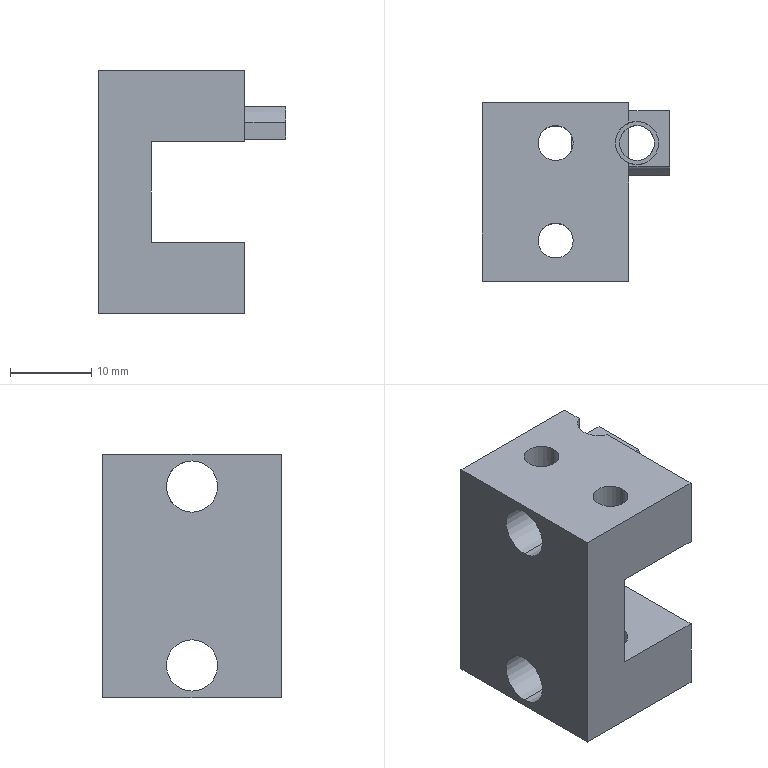Part | SolidWorks | features BaseBody 1 | 1 solid | 36 faces | box 23 x 22 x 30 mm | volume 7166 mm3 | plane 20 | cylinder 16 | commonest cylinder face diameters 4.3 x10 6.3 x4 5.3 x2
STEP:
#1=CARTESIAN_POINT('',(-9.,0.,7.85));
#2=VERTEX_POINT('',#1);
#3=CARTESIAN_POINT('',(-9.,0.,14.15));
#4=VERTEX_POINT('',#3);
#5=CARTESIAN_POINT('',(-9.,0.,11.));
#6=DIRECTION('',(-1.,0.,0.));
#7=DIRECTION('',(0.,0.,-1.));
#8=AXIS2_PLACEMENT_3D('',#5,#6,#7);
#9=CIRCLE('',#8,3.15);
#10=EDGE_CURVE('',#2,#4,#9,.T.);
#11=ORIENTED_EDGE('',*,*,#10,.T.);
#12=CARTESIAN_POINT('',(9.,0.,14.15));
#13=VERTEX_POINT('',#12);
#14=CARTESIAN_POINT('',(-10.,0.,14.15));
#15=DIRECTION('',(1.,0.,0.));
#16=VECTOR('',#15,1000.);
#17=LINE('',#14,#16);
#18=EDGE_CURVE('',#4,#13,#17,.T.);
#19=ORIENTED_EDGE('',*,*,#18,.T.);
#20=CARTESIAN_POINT('',(9.,0.,7.85));
#21=VERTEX_POINT('',#20);
#22=CARTESIAN_POINT('',(9.,0.,11.));
#23=DIRECTION('',(-1.,0.,0.));
#24=DIRECTION('',(0.,0.,-1.));
#25=AXIS2_PLACEMENT_3D('',#22,#23,#24);
#26=CIRCLE('',#25,3.15);
#27=EDGE_CURVE('',#21,#13,#26,.T.);
#28=ORIENTED_EDGE('',*,*,#27,.F.);
#29=CARTESIAN_POINT('',(-10.,0.,7.85));
#30=DIRECTION('',(1.,0.,0.));
#31=VECTOR('',#30,1000.);
#32=LINE('',#29,#31);
#33=EDGE_CURVE('',#2,#21,#32,.T.);
#34=ORIENTED_EDGE('',*,*,#33,.F.);
#35=EDGE_LOOP('',(#11,#19,#28,#34));
#36=FACE_OUTER_BOUND('',#35,.T.);
#37=CARTESIAN_POINT('',(-10.,0.,11.));
#38=DIRECTION('',(1.,0.,0.));
#39=DIRECTION('',(0.,0.,-1.));
#40=AXIS2_PLACEMENT_3D('',#37,#38,#39);
#41=CYLINDRICAL_SURFACE('',#40,3.15);
#42=ADVANCED_FACE('',(#36),#41,.F.);
#43=CARTESIAN_POINT('',(-9.,0.,-14.15));
#44=VERTEX_POINT('',#43);
#45=CARTESIAN_POINT('',(-9.,0.,-7.85));
#46=VERTEX_POINT('',#45);
#47=CARTESIAN_POINT('',(-9.,0.,-11.));
#48=DIRECTION('',(-1.,0.,0.));
#49=DIRECTION('',(0.,0.,-1.));
#50=AXIS2_PLACEMENT_3D('',#47,#48,#49);
#51=CIRCLE('',#50,3.15);
#52=EDGE_CURVE('',#44,#46,#51,.T.);
#53=ORIENTED_EDGE('',*,*,#52,.T.);
#54=CARTESIAN_POINT('',(9.,0.,-7.85));
#55=VERTEX_POINT('',#54);
#56=CARTESIAN_POINT('',(-10.,0.,-7.85));
#57=DIRECTION('',(1.,0.,0.));
#58=VECTOR('',#57,1000.);
#59=LINE('',#56,#58);
#60=EDGE_CURVE('',#46,#55,#59,.T.);
#61=ORIENTED_EDGE('',*,*,#60,.T.);
#62=CARTESIAN_POINT('',(9.,0.,-14.15));
#63=VERTEX_POINT('',#62);
#64=CARTESIAN_POINT('',(9.,0.,-11.));
#65=DIRECTION('',(-1.,0.,0.));
#66=DIRECTION('',(0.,0.,-1.));
#67=AXIS2_PLACEMENT_3D('',#64,#65,#66);
#68=CIRCLE('',#67,3.15);
#69=EDGE_CURVE('',#63,#55,#68,.T.);
#70=ORIENTED_EDGE('',*,*,#69,.F.);
#71=CARTESIAN_POINT('',(-10.,0.,-14.15));
#72=DIRECTION('',(1.,0.,0.));
#73=VECTOR('',#72,1000.);
#74=LINE('',#71,#73);
#75=EDGE_CURVE('',#44,#63,#74,.T.);
#76=ORIENTED_EDGE('',*,*,#75,.F.);
#77=EDGE_LOOP('',(#53,#61,#70,#76));
#78=FACE_OUTER_BOUND('',#77,.T.);
#79=CARTESIAN_POINT('',(-10.,0.,-11.));
#80=DIRECTION('',(1.,0.,0.));
#81=DIRECTION('',(0.,0.,-1.));
#82=AXIS2_PLACEMENT_3D('',#79,#80,#81);
#83=CYLINDRICAL_SURFACE('',#82,3.15);
#84=ADVANCED_FACE('',(#78),#83,.F.);
#85=CARTESIAN_POINT('',(-2.15,6.,6.2));
#86=VERTEX_POINT('',#85);
#87=CARTESIAN_POINT('',(2.15,6.,6.2));
#88=VERTEX_POINT('',#87);
#89=CARTESIAN_POINT('',(0.,6.,6.2));
#90=DIRECTION('',(0.,0.,1.));
#91=DIRECTION('',(1.,0.,0.));
#92=AXIS2_PLACEMENT_3D('',#89,#90,#91);
#93=CIRCLE('',#92,2.15);
#94=EDGE_CURVE('',#86,#88,#93,.T.);
#95=ORIENTED_EDGE('',*,*,#94,.F.);
#96=CARTESIAN_POINT('',(-2.15,6.,15.));
#97=VERTEX_POINT('',#96);
#98=CARTESIAN_POINT('',(-2.15,6.,-16.));
#99=DIRECTION('',(0.,0.,1.));
#100=VECTOR('',#99,1000.);
#101=LINE('',#98,#100);
#102=EDGE_CURVE('',#86,#97,#101,.T.);
#103=ORIENTED_EDGE('',*,*,#102,.T.);
#104=CARTESIAN_POINT('',(2.15,6.,15.));
#105=VERTEX_POINT('',#104);
#106=CARTESIAN_POINT('',(0.,6.,15.));
#107=DIRECTION('',(0.,0.,-1.));
#108=DIRECTION('',(1.,0.,0.));
#109=AXIS2_PLACEMENT_3D('',#106,#107,#108);
#110=CIRCLE('',#109,2.15);
#111=EDGE_CURVE('',#105,#97,#110,.T.);
#112=ORIENTED_EDGE('',*,*,#111,.F.);
#113=CARTESIAN_POINT('',(2.15,6.,10.5));
#114=VERTEX_POINT('',#113);
#115=CARTESIAN_POINT('',(2.15,6.,-16.));
#116=DIRECTION('',(0.,0.,1.));
#117=VECTOR('',#116,1000.);
#118=LINE('',#115,#117);
#119=EDGE_CURVE('',#114,#105,#118,.T.);
#120=ORIENTED_EDGE('',*,*,#119,.F.);
#121=CARTESIAN_POINT('',(2.,5.211,10.5));
#122=VERTEX_POINT('',#121);
#123=CARTESIAN_POINT('',(0.,6.,10.5));
#124=DIRECTION('',(0.,0.,1.));
#125=DIRECTION('',(1.,0.,0.));
#126=AXIS2_PLACEMENT_3D('',#123,#124,#125);
#127=CIRCLE('',#126,2.15);
#128=EDGE_CURVE('',#122,#114,#127,.T.);
#129=ORIENTED_EDGE('',*,*,#128,.F.);
#130=CARTESIAN_POINT('',(2.,5.211,6.5));
#131=VERTEX_POINT('',#130);
#132=CARTESIAN_POINT('',(2.,5.211,-16.));
#133=DIRECTION('',(0.,0.,1.));
#134=VECTOR('',#133,1000.);
#135=LINE('',#132,#134);
#136=EDGE_CURVE('',#131,#122,#135,.T.);
#137=ORIENTED_EDGE('',*,*,#136,.F.);
#138=CARTESIAN_POINT('',(2.15,6.,6.5));
#139=VERTEX_POINT('',#138);
#140=CARTESIAN_POINT('',(0.,6.,6.5));
#141=DIRECTION('',(0.,0.,-1.));
#142=DIRECTION('',(1.,0.,0.));
#143=AXIS2_PLACEMENT_3D('',#140,#141,#142);
#144=CIRCLE('',#143,2.15);
#145=EDGE_CURVE('',#139,#131,#144,.T.);
#146=ORIENTED_EDGE('',*,*,#145,.F.);
#147=CARTESIAN_POINT('',(2.15,6.,-16.));
#148=DIRECTION('',(0.,0.,1.));
#149=VECTOR('',#148,1000.);
#150=LINE('',#147,#149);
#151=EDGE_CURVE('',#88,#139,#150,.T.);
#152=ORIENTED_EDGE('',*,*,#151,.F.);
#153=EDGE_LOOP('',(#95,#103,#112,#120,#129,#137,#146,#152));
#154=FACE_OUTER_BOUND('',#153,.T.);
#155=CARTESIAN_POINT('',(0.,6.,-16.));
#156=DIRECTION('',(0.,0.,1.));
#157=DIRECTION('',(1.,0.,0.));
#158=AXIS2_PLACEMENT_3D('',#155,#156,#157);
#159=CYLINDRICAL_SURFACE('',#158,2.15);
#160=ADVANCED_FACE('',(#154),#159,.F.);
#161=CARTESIAN_POINT('',(-2.15,-6.,6.2));
#162=VERTEX_POINT('',#161);
#163=CARTESIAN_POINT('',(2.15,-6.,6.2));
#164=VERTEX_POINT('',#163);
#165=CARTESIAN_POINT('',(0.,-6.,6.2));
#166=DIRECTION('',(0.,0.,1.));
#167=DIRECTION('',(1.,0.,0.));
#168=AXIS2_PLACEMENT_3D('',#165,#166,#167);
#169=CIRCLE('',#168,2.15);
#170=EDGE_CURVE('',#162,#164,#169,.T.);
#171=ORIENTED_EDGE('',*,*,#170,.F.);
#172=CARTESIAN_POINT('',(-2.15,-6.,15.));
#173=VERTEX_POINT('',#172);
#174=CARTESIAN_POINT('',(-2.15,-6.,-16.));
#175=DIRECTION('',(0.,0.,1.));
#176=VECTOR('',#175,1000.);
#177=LINE('',#174,#176);
#178=EDGE_CURVE('',#162,#173,#177,.T.);
#179=ORIENTED_EDGE('',*,*,#178,.T.);
#180=CARTESIAN_POINT('',(2.15,-6.,15.));
#181=VERTEX_POINT('',#180);
#182=CARTESIAN_POINT('',(0.,-6.,15.));
#183=DIRECTION('',(0.,0.,-1.));
#184=DIRECTION('',(1.,0.,0.));
#185=AXIS2_PLACEMENT_3D('',#182,#183,#184);
#186=CIRCLE('',#185,2.15);
#187=EDGE_CURVE('',#181,#173,#186,.T.);
#188=ORIENTED_EDGE('',*,*,#187,.F.);
#189=CARTESIAN_POINT('',(2.15,-6.,-16.));
#190=DIRECTION('',(0.,0.,1.));
#191=VECTOR('',#190,1000.);
#192=LINE('',#189,#191);
#193=EDGE_CURVE('',#164,#181,#192,.T.);
#194=ORIENTED_EDGE('',*,*,#193,.F.);
#195=EDGE_LOOP('',(#171,#179,#188,#194));
#196=FACE_OUTER_BOUND('',#195,.T.);
#197=CARTESIAN_POINT('',(0.,-6.,-16.));
#198=DIRECTION('',(0.,0.,1.));
#199=DIRECTION('',(1.,0.,0.));
#200=AXIS2_PLACEMENT_3D('',#197,#198,#199);
#201=CYLINDRICAL_SURFACE('',#200,2.15);
#202=ADVANCED_FACE('',(#196),#201,.F.);
#203=CARTESIAN_POINT('',(7.35,6.,9.));
#204=VERTEX_POINT('',#203);
#205=CARTESIAN_POINT('',(12.65,6.,9.));
#206=VERTEX_POINT('',#205);
#207=CARTESIAN_POINT('',(10.,6.,9.));
#208=DIRECTION('',(0.,0.,1.));
#209=DIRECTION('',(1.,0.,0.));
#210=AXIS2_PLACEMENT_3D('',#207,#208,#209);
#211=CIRCLE('',#210,2.65);
#212=EDGE_CURVE('',#204,#206,#211,.T.);
#213=ORIENTED_EDGE('',*,*,#212,.F.);
#214=CARTESIAN_POINT('',(7.35,6.,15.));
#215=VERTEX_POINT('',#214);
#216=CARTESIAN_POINT('',(7.35,6.,9.));
#217=DIRECTION('',(0.,0.,1.));
#218=VECTOR('',#217,1000.);
#219=LINE('',#216,#218);
#220=EDGE_CURVE('',#204,#215,#219,.T.);
#221=ORIENTED_EDGE('',*,*,#220,.T.);
#222=CARTESIAN_POINT('',(9.,3.546,15.));
#223=VERTEX_POINT('',#222);
#224=CARTESIAN_POINT('',(10.,6.,15.));
#225=DIRECTION('',(0.,0.,-1.));
#226=DIRECTION('',(1.,0.,0.));
#227=AXIS2_PLACEMENT_3D('',#224,#225,#226);
#228=CIRCLE('',#227,2.65);
#229=EDGE_CURVE('',#223,#215,#228,.T.);
#230=ORIENTED_EDGE('',*,*,#229,.F.);
#231=CARTESIAN_POINT('',(9.,3.546,10.5));
#232=VERTEX_POINT('',#231);
#233=CARTESIAN_POINT('',(9.,3.546,-15.));
#234=DIRECTION('',(0.,0.,1.));
#235=VECTOR('',#234,1000.);
#236=LINE('',#233,#235);
#237=EDGE_CURVE('',#232,#223,#236,.T.);
#238=ORIENTED_EDGE('',*,*,#237,.F.);
#239=CARTESIAN_POINT('',(12.65,6.,10.5));
#240=VERTEX_POINT('',#239);
#241=CARTESIAN_POINT('',(10.,6.,10.5));
#242=DIRECTION('',(0.,0.,-1.));
#243=DIRECTION('',(1.,0.,0.));
#244=AXIS2_PLACEMENT_3D('',#241,#242,#243);
#245=CIRCLE('',#244,2.65);
#246=EDGE_CURVE('',#240,#232,#245,.T.);
#247=ORIENTED_EDGE('',*,*,#246,.F.);
#248=CARTESIAN_POINT('',(12.65,6.,9.));
#249=DIRECTION('',(0.,0.,1.));
#250=VECTOR('',#249,1000.);
#251=LINE('',#248,#250);
#252=EDGE_CURVE('',#206,#240,#251,.T.);
#253=ORIENTED_EDGE('',*,*,#252,.F.);
#254=EDGE_LOOP('',(#213,#221,#230,#238,#247,#253));
#255=FACE_OUTER_BOUND('',#254,.T.);
#256=CARTESIAN_POINT('',(10.,6.,9.));
#257=DIRECTION('',(0.,0.,1.));
#258=DIRECTION('',(1.,0.,0.));
#259=AXIS2_PLACEMENT_3D('',#256,#257,#258);
#260=CYLINDRICAL_SURFACE('',#259,2.65);
#261=ADVANCED_FACE('',(#255),#260,.F.);
#262=CARTESIAN_POINT('',(2.15,6.,-15.));
#263=VERTEX_POINT('',#262);
#264=CARTESIAN_POINT('',(-2.15,6.,-15.));
#265=VERTEX_POINT('',#264);
#266=CARTESIAN_POINT('',(0.,6.,-15.));
#267=DIRECTION('',(0.,0.,-1.));
#268=DIRECTION('',(1.,0.,0.));
#269=AXIS2_PLACEMENT_3D('',#266,#267,#268);
#270=CIRCLE('',#269,2.15);
#271=EDGE_CURVE('',#263,#265,#270,.T.);
#272=ORIENTED_EDGE('',*,*,#271,.T.);
#273=CARTESIAN_POINT('',(-2.15,6.,-6.2));
#274=VERTEX_POINT('',#273);
#275=CARTESIAN_POINT('',(-2.15,6.,-16.));
#276=DIRECTION('',(0.,0.,1.));
#277=VECTOR('',#276,1000.);
#278=LINE('',#275,#277);
#279=EDGE_CURVE('',#265,#274,#278,.T.);
#280=ORIENTED_EDGE('',*,*,#279,.T.);
#281=CARTESIAN_POINT('',(2.15,6.,-6.2));
#282=VERTEX_POINT('',#281);
#283=CARTESIAN_POINT('',(0.,6.,-6.2));
#284=DIRECTION('',(0.,0.,-1.));
#285=DIRECTION('',(1.,0.,0.));
#286=AXIS2_PLACEMENT_3D('',#283,#284,#285);
#287=CIRCLE('',#286,2.15);
#288=EDGE_CURVE('',#282,#274,#287,.T.);
#289=ORIENTED_EDGE('',*,*,#288,.F.);
#290=CARTESIAN_POINT('',(2.15,6.,-16.));
#291=DIRECTION('',(0.,0.,1.));
#292=VECTOR('',#291,1000.);
#293=LINE('',#290,#292);
#294=EDGE_CURVE('',#263,#282,#293,.T.);
#295=ORIENTED_EDGE('',*,*,#294,.F.);
#296=EDGE_LOOP('',(#272,#280,#289,#295));
#297=FACE_OUTER_BOUND('',#296,.T.);
#298=CARTESIAN_POINT('',(0.,6.,-16.));
#299=DIRECTION('',(0.,0.,1.));
#300=DIRECTION('',(1.,0.,0.));
#301=AXIS2_PLACEMENT_3D('',#298,#299,#300);
#302=CYLINDRICAL_SURFACE('',#301,2.15);
#303=ADVANCED_FACE('',(#297),#302,.F.);
#304=CARTESIAN_POINT('',(2.15,-6.,-15.));
#305=VERTEX_POINT('',#304);
#306=CARTESIAN_POINT('',(-2.15,-6.,-15.));
#307=VERTEX_POINT('',#306);
#308=CARTESIAN_POINT('',(0.,-6.,-15.));
#309=DIRECTION('',(0.,0.,-1.));
#310=DIRECTION('',(1.,0.,0.));
#311=AXIS2_PLACEMENT_3D('',#308,#309,#310);
#312=CIRCLE('',#311,2.15);
#313=EDGE_CURVE('',#305,#307,#312,.T.);
#314=ORIENTED_EDGE('',*,*,#313,.T.);
#315=CARTESIAN_POINT('',(-2.15,-6.,-6.2));
#316=VERTEX_POINT('',#315);
#317=CARTESIAN_POINT('',(-2.15,-6.,-16.));
#318=DIRECTION('',(0.,0.,1.));
#319=VECTOR('',#318,1000.);
#320=LINE('',#317,#319);
#321=EDGE_CURVE('',#307,#316,#320,.T.);
#322=ORIENTED_EDGE('',*,*,#321,.T.);
#323=CARTESIAN_POINT('',(2.15,-6.,-6.2));
#324=VERTEX_POINT('',#323);
#325=CARTESIAN_POINT('',(0.,-6.,-6.2));
#326=DIRECTION('',(0.,0.,-1.));
#327=DIRECTION('',(1.,0.,0.));
#328=AXIS2_PLACEMENT_3D('',#325,#326,#327);
#329=CIRCLE('',#328,2.15);
#330=EDGE_CURVE('',#324,#316,#329,.T.);
#331=ORIENTED_EDGE('',*,*,#330,.F.);
#332=CARTESIAN_POINT('',(2.15,-6.,-16.));
#333=DIRECTION('',(0.,0.,1.));
#334=VECTOR('',#333,1000.);
#335=LINE('',#332,#334);
#336=EDGE_CURVE('',#305,#324,#335,.T.);
#337=ORIENTED_EDGE('',*,*,#336,.F.);
#338=EDGE_LOOP('',(#314,#322,#331,#337));
#339=FACE_OUTER_BOUND('',#338,.T.);
#340=CARTESIAN_POINT('',(0.,-6.,-16.));
#341=DIRECTION('',(0.,0.,1.));
#342=DIRECTION('',(1.,0.,0.));
#343=AXIS2_PLACEMENT_3D('',#340,#341,#342);
#344=CYLINDRICAL_SURFACE('',#343,2.15);
#345=ADVANCED_FACE('',(#339),#344,.F.);
#346=CARTESIAN_POINT('',(9.,4.097,6.2));
#347=VERTEX_POINT('',#346);
#348=CARTESIAN_POINT('',(7.85,6.,6.2));
#349=VERTEX_POINT('',#348);
#350=CARTESIAN_POINT('',(10.,6.,6.2));
#351=DIRECTION('',(0.,0.,-1.));
#352=DIRECTION('',(1.,0.,0.));
#353=AXIS2_PLACEMENT_3D('',#350,#351,#352);
#354=CIRCLE('',#353,2.15);
#355=EDGE_CURVE('',#347,#349,#354,.T.);
#356=ORIENTED_EDGE('',*,*,#355,.T.);
#357=CARTESIAN_POINT('',(7.85,6.,9.));
#358=VERTEX_POINT('',#357);
#359=CARTESIAN_POINT('',(7.85,6.,0.5));
#360=DIRECTION('',(0.,0.,1.));
#361=VECTOR('',#360,1000.);
#362=LINE('',#359,#361);
#363=EDGE_CURVE('',#349,#358,#362,.T.);
#364=ORIENTED_EDGE('',*,*,#363,.T.);
#365=CARTESIAN_POINT('',(12.15,6.,9.));
#366=VERTEX_POINT('',#365);
#367=CARTESIAN_POINT('',(10.,6.,9.));
#368=DIRECTION('',(0.,0.,-1.));
#369=DIRECTION('',(1.,0.,0.));
#370=AXIS2_PLACEMENT_3D('',#367,#368,#369);
#371=CIRCLE('',#370,2.15);
#372=EDGE_CURVE('',#366,#358,#371,.T.);
#373=ORIENTED_EDGE('',*,*,#372,.F.);
#374=CARTESIAN_POINT('',(12.15,6.,6.5));
#375=VERTEX_POINT('',#374);
#376=CARTESIAN_POINT('',(12.15,6.,0.5));
#377=DIRECTION('',(0.,0.,1.));
#378=VECTOR('',#377,1000.);
#379=LINE('',#376,#378);
#380=EDGE_CURVE('',#375,#366,#379,.T.);
#381=ORIENTED_EDGE('',*,*,#380,.F.);
#382=CARTESIAN_POINT('',(9.,4.097,6.5));
#383=VERTEX_POINT('',#382);
#384=CARTESIAN_POINT('',(10.,6.,6.5));
#385=DIRECTION('',(0.,0.,-1.));
#386=DIRECTION('',(1.,0.,0.));
#387=AXIS2_PLACEMENT_3D('',#384,#385,#386);
#388=CIRCLE('',#387,2.15);
#389=EDGE_CURVE('',#375,#383,#388,.T.);
#390=ORIENTED_EDGE('',*,*,#389,.T.);
#391=CARTESIAN_POINT('',(9.,4.097,0.5));
#392=DIRECTION('',(0.,0.,1.));
#393=VECTOR('',#392,1000.);
#394=LINE('',#391,#393);
#395=EDGE_CURVE('',#347,#383,#394,.T.);
#396=ORIENTED_EDGE('',*,*,#395,.F.);
#397=EDGE_LOOP('',(#356,#364,#373,#381,#390,#396));
#398=FACE_OUTER_BOUND('',#397,.T.);
#399=CARTESIAN_POINT('',(10.,6.,0.5));
#400=DIRECTION('',(0.,0.,1.));
#401=DIRECTION('',(1.,0.,0.));
#402=AXIS2_PLACEMENT_3D('',#399,#400,#401);
#403=CYLINDRICAL_SURFACE('',#402,2.15);
#404=ADVANCED_FACE('',(#398),#403,.F.);
#405=ORIENTED_EDGE('',*,*,#10,.F.);
#406=CARTESIAN_POINT('',(-9.,0.,11.));
#407=DIRECTION('',(-1.,0.,0.));
#408=DIRECTION('',(0.,0.,-1.));
#409=AXIS2_PLACEMENT_3D('',#406,#407,#408);
#410=CIRCLE('',#409,3.15);
#411=EDGE_CURVE('',#4,#2,#410,.T.);
#412=ORIENTED_EDGE('',*,*,#411,.F.);
#413=EDGE_LOOP('',(#405,#412));
#414=FACE_BOUND('',#413,.T.);
#415=ORIENTED_EDGE('',*,*,#52,.F.);
#416=CARTESIAN_POINT('',(-9.,0.,-11.));
#417=DIRECTION('',(-1.,0.,0.));
#418=DIRECTION('',(0.,0.,-1.));
#419=AXIS2_PLACEMENT_3D('',#416,#417,#418);
#420=CIRCLE('',#419,3.15);
#421=EDGE_CURVE('',#46,#44,#420,.T.);
#422=ORIENTED_EDGE('',*,*,#421,.F.);
#423=EDGE_LOOP('',(#415,#422));
#424=FACE_BOUND('',#423,.T.);
#425=CARTESIAN_POINT('',(-9.,11.,-15.));
#426=VERTEX_POINT('',#425);
#427=CARTESIAN_POINT('',(-9.,11.,15.));
#428=VERTEX_POINT('',#427);
#429=CARTESIAN_POINT('',(-9.,11.,-15.));
#430=DIRECTION('',(0.,0.,1.));
#431=VECTOR('',#430,1000.);
#432=LINE('',#429,#431);
#433=EDGE_CURVE('',#426,#428,#432,.T.);
#434=ORIENTED_EDGE('',*,*,#433,.F.);
#435=CARTESIAN_POINT('',(-9.,-11.,-15.));
#436=VERTEX_POINT('',#435);
#437=CARTESIAN_POINT('',(-9.,-11.,-15.));
#438=DIRECTION('',(0.,1.,0.));
#439=VECTOR('',#438,1000.);
#440=LINE('',#437,#439);
#441=EDGE_CURVE('',#436,#426,#440,.T.);
#442=ORIENTED_EDGE('',*,*,#441,.F.);
#443=CARTESIAN_POINT('',(-9.,-11.,15.));
#444=VERTEX_POINT('',#443);
#445=CARTESIAN_POINT('',(-9.,-11.,-15.));
#446=DIRECTION('',(0.,0.,-1.));
#447=VECTOR('',#446,1000.);
#448=LINE('',#445,#447);
#449=EDGE_CURVE('',#444,#436,#448,.T.);
#450=ORIENTED_EDGE('',*,*,#449,.F.);
#451=CARTESIAN_POINT('',(-9.,-11.,15.));
#452=DIRECTION('',(0.,-1.,0.));
#453=VECTOR('',#452,1000.);
#454=LINE('',#451,#453);
#455=EDGE_CURVE('',#428,#444,#454,.T.);
#456=ORIENTED_EDGE('',*,*,#455,.F.);
#457=EDGE_LOOP('',(#434,#442,#450,#456));
#458=FACE_OUTER_BOUND('',#457,.T.);
#459=CARTESIAN_POINT('',(-9.,-11.,-15.));
#460=DIRECTION('',(1.,0.,0.));
#461=DIRECTION('',(0.,0.,-1.));
#462=AXIS2_PLACEMENT_3D('',#459,#460,#461);
#463=PLANE('',#462);
#464=ADVANCED_FACE('',(#414,#424,#458),#463,.F.);
#465=ORIENTED_EDGE('',*,*,#18,.F.);
#466=ORIENTED_EDGE('',*,*,#411,.T.);
#467=ORIENTED_EDGE('',*,*,#33,.T.);
#468=CARTESIAN_POINT('',(9.,2.,8.566));
#469=VERTEX_POINT('',#468);
#470=CARTESIAN_POINT('',(9.,0.,11.));
#471=DIRECTION('',(-1.,0.,0.));
#472=DIRECTION('',(0.,0.,-1.));
#473=AXIS2_PLACEMENT_3D('',#470,#471,#472);
#474=CIRCLE('',#473,3.15);
#475=EDGE_CURVE('',#469,#21,#474,.T.);
#476=ORIENTED_EDGE('',*,*,#475,.F.);
#477=CARTESIAN_POINT('',(14.,2.,8.566));
#478=VERTEX_POINT('',#477);
#479=CARTESIAN_POINT('',(-10.,2.,8.566));
#480=DIRECTION('',(-1.,0.,0.));
#481=VECTOR('',#480,1000.);
#482=LINE('',#479,#481);
#483=EDGE_CURVE('',#478,#469,#482,.T.);
#484=ORIENTED_EDGE('',*,*,#483,.F.);
#485=CARTESIAN_POINT('',(14.,3.11,10.5));
#486=VERTEX_POINT('',#485);
#487=CARTESIAN_POINT('',(14.,0.,11.));
#488=DIRECTION('',(-1.,0.,0.));
#489=DIRECTION('',(0.,0.,-1.));
#490=AXIS2_PLACEMENT_3D('',#487,#488,#489);
#491=CIRCLE('',#490,3.15);
#492=EDGE_CURVE('',#486,#478,#491,.T.);
#493=ORIENTED_EDGE('',*,*,#492,.F.);
#494=CARTESIAN_POINT('',(9.,3.11,10.5));
#495=VERTEX_POINT('',#494);
#496=CARTESIAN_POINT('',(-10.,3.11,10.5));
#497=DIRECTION('',(1.,0.,0.));
#498=VECTOR('',#497,1000.);
#499=LINE('',#496,#498);
#500=EDGE_CURVE('',#495,#486,#499,.T.);
#501=ORIENTED_EDGE('',*,*,#500,.F.);
#502=CARTESIAN_POINT('',(9.,0.,11.));
#503=DIRECTION('',(-1.,0.,0.));
#504=DIRECTION('',(0.,0.,-1.));
#505=AXIS2_PLACEMENT_3D('',#502,#503,#504);
#506=CIRCLE('',#505,3.15);
#507=EDGE_CURVE('',#13,#495,#506,.T.);
#508=ORIENTED_EDGE('',*,*,#507,.F.);
#509=EDGE_LOOP('',(#465,#466,#467,#476,#484,#493,#501,#508));
#510=FACE_OUTER_BOUND('',#509,.T.);
#511=CARTESIAN_POINT('',(-10.,0.,11.));
#512=DIRECTION('',(1.,0.,0.));
#513=DIRECTION('',(0.,0.,-1.));
#514=AXIS2_PLACEMENT_3D('',#511,#512,#513);
#515=CYLINDRICAL_SURFACE('',#514,3.15);
#516=ADVANCED_FACE('',(#510),#515,.F.);
#517=ORIENTED_EDGE('',*,*,#60,.F.);
#518=ORIENTED_EDGE('',*,*,#421,.T.);
#519=ORIENTED_EDGE('',*,*,#75,.T.);
#520=CARTESIAN_POINT('',(9.,0.,-11.));
#521=DIRECTION('',(-1.,0.,0.));
#522=DIRECTION('',(0.,0.,-1.));
#523=AXIS2_PLACEMENT_3D('',#520,#521,#522);
#524=CIRCLE('',#523,3.15);
#525=EDGE_CURVE('',#55,#63,#524,.T.);
#526=ORIENTED_EDGE('',*,*,#525,.F.);
#527=EDGE_LOOP('',(#517,#518,#519,#526));
#528=FACE_OUTER_BOUND('',#527,.T.);
#529=CARTESIAN_POINT('',(-10.,0.,-11.));
#530=DIRECTION('',(1.,0.,0.));
#531=DIRECTION('',(0.,0.,-1.));
#532=AXIS2_PLACEMENT_3D('',#529,#530,#531);
#533=CYLINDRICAL_SURFACE('',#532,3.15);
#534=ADVANCED_FACE('',(#528),#533,.F.);
#535=ORIENTED_EDGE('',*,*,#111,.T.);
#536=CARTESIAN_POINT('',(0.,6.,15.));
#537=DIRECTION('',(0.,0.,-1.));
#538=DIRECTION('',(1.,0.,0.));
#539=AXIS2_PLACEMENT_3D('',#536,#537,#538);
#540=CIRCLE('',#539,2.15);
#541=EDGE_CURVE('',#97,#105,#540,.T.);
#542=ORIENTED_EDGE('',*,*,#541,.T.);
#543=EDGE_LOOP('',(#535,#542));
#544=FACE_BOUND('',#543,.T.);
#545=ORIENTED_EDGE('',*,*,#187,.T.);
#546=CARTESIAN_POINT('',(0.,-6.,15.));
#547=DIRECTION('',(0.,0.,-1.));
#548=DIRECTION('',(1.,0.,0.));
#549=AXIS2_PLACEMENT_3D('',#546,#547,#548);
#550=CIRCLE('',#549,2.15);
#551=EDGE_CURVE('',#173,#181,#550,.T.);
#552=ORIENTED_EDGE('',*,*,#551,.T.);
#553=EDGE_LOOP('',(#545,#552));
#554=FACE_BOUND('',#553,.T.);
#555=ORIENTED_EDGE('',*,*,#229,.T.);
#556=CARTESIAN_POINT('',(9.,8.454,15.));
#557=VERTEX_POINT('',#556);
#558=CARTESIAN_POINT('',(10.,6.,15.));
#559=DIRECTION('',(0.,0.,-1.));
#560=DIRECTION('',(1.,0.,0.));
#561=AXIS2_PLACEMENT_3D('',#558,#559,#560);
#562=CIRCLE('',#561,2.65);
#563=EDGE_CURVE('',#215,#557,#562,.T.);
#564=ORIENTED_EDGE('',*,*,#563,.T.);
#565=CARTESIAN_POINT('',(9.,11.,15.));
#566=VERTEX_POINT('',#565);
#567=CARTESIAN_POINT('',(9.,-11.,15.));
#568=DIRECTION('',(0.,1.,0.));
#569=VECTOR('',#568,1000.);
#570=LINE('',#567,#569);
#571=EDGE_CURVE('',#557,#566,#570,.T.);
#572=ORIENTED_EDGE('',*,*,#571,.T.);
#573=CARTESIAN_POINT('',(-9.,11.,15.));
#574=DIRECTION('',(-1.,0.,0.));
#575=VECTOR('',#574,1000.);
#576=LINE('',#573,#575);
#577=EDGE_CURVE('',#566,#428,#576,.T.);
#578=ORIENTED_EDGE('',*,*,#577,.T.);
#579=ORIENTED_EDGE('',*,*,#455,.T.);
#580=CARTESIAN_POINT('',(9.,-11.,15.));
#581=VERTEX_POINT('',#580);
#582=CARTESIAN_POINT('',(-9.,-11.,15.));
#583=DIRECTION('',(1.,0.,0.));
#584=VECTOR('',#583,1000.);
#585=LINE('',#582,#584);
#586=EDGE_CURVE('',#444,#581,#585,.T.);
#587=ORIENTED_EDGE('',*,*,#586,.T.);
#588=CARTESIAN_POINT('',(9.,-11.,15.));
#589=DIRECTION('',(0.,1.,0.));
#590=VECTOR('',#589,1000.);
#591=LINE('',#588,#590);
#592=EDGE_CURVE('',#581,#223,#591,.T.);
#593=ORIENTED_EDGE('',*,*,#592,.T.);
#594=EDGE_LOOP('',(#555,#564,#572,#578,#579,#587,#593));
#595=FACE_OUTER_BOUND('',#594,.T.);
#596=CARTESIAN_POINT('',(-9.,-11.,15.));
#597=DIRECTION('',(0.,0.,1.));
#598=DIRECTION('',(1.,0.,0.));
#599=AXIS2_PLACEMENT_3D('',#596,#597,#598);
#600=PLANE('',#599);
#601=ADVANCED_FACE('',(#544,#554,#595),#600,.T.);
#602=CARTESIAN_POINT('',(-2.5,11.,6.2));
#603=VERTEX_POINT('',#602);
#604=CARTESIAN_POINT('',(-2.5,11.,-6.2));
#605=VERTEX_POINT('',#604);
#606=CARTESIAN_POINT('',(-2.5,11.,-15.));
#607=DIRECTION('',(0.,0.,-1.));
#608=VECTOR('',#607,1000.);
#609=LINE('',#606,#608);
#610=EDGE_CURVE('',#603,#605,#609,.T.);
#611=ORIENTED_EDGE('',*,*,#610,.T.);
#612=CARTESIAN_POINT('',(9.,11.,-6.2));
#613=VERTEX_POINT('',#612);
#614=CARTESIAN_POINT('',(-9.,11.,-6.2));
#615=DIRECTION('',(1.,0.,0.));
#616=VECTOR('',#615,1000.);
#617=LINE('',#614,#616);
#618=EDGE_CURVE('',#605,#613,#617,.T.);
#619=ORIENTED_EDGE('',*,*,#618,.T.);
#620=CARTESIAN_POINT('',(9.,11.,-15.));
#621=VERTEX_POINT('',#620);
#622=CARTESIAN_POINT('',(9.,11.,-15.));
#623=DIRECTION('',(0.,0.,-1.));
#624=VECTOR('',#623,1000.);
#625=LINE('',#622,#624);
#626=EDGE_CURVE('',#613,#621,#625,.T.);
#627=ORIENTED_EDGE('',*,*,#626,.T.);
#628=CARTESIAN_POINT('',(-9.,11.,-15.));
#629=DIRECTION('',(-1.,0.,0.));
#630=VECTOR('',#629,1000.);
#631=LINE('',#628,#630);
#632=EDGE_CURVE('',#621,#426,#631,.T.);
#633=ORIENTED_EDGE('',*,*,#632,.T.);
#634=ORIENTED_EDGE('',*,*,#433,.T.);
#635=ORIENTED_EDGE('',*,*,#577,.F.);
#636=CARTESIAN_POINT('',(9.,11.,6.2));
#637=VERTEX_POINT('',#636);
#638=CARTESIAN_POINT('',(9.,11.,-15.));
#639=DIRECTION('',(0.,0.,-1.));
#640=VECTOR('',#639,1000.);
#641=LINE('',#638,#640);
#642=EDGE_CURVE('',#566,#637,#641,.T.);
#643=ORIENTED_EDGE('',*,*,#642,.T.);
#644=CARTESIAN_POINT('',(-9.,11.,6.2));
#645=DIRECTION('',(-1.,0.,0.));
#646=VECTOR('',#645,1000.);
#647=LINE('',#644,#646);
#648=EDGE_CURVE('',#637,#603,#647,.T.);
#649=ORIENTED_EDGE('',*,*,#648,.T.);
#650=EDGE_LOOP('',(#611,#619,#627,#633,#634,#635,#643,#649));
#651=FACE_OUTER_BOUND('',#650,.T.);
#652=CARTESIAN_POINT('',(-9.,11.,-15.));
#653=DIRECTION('',(0.,1.,0.));
#654=DIRECTION('',(0.,0.,1.));
#655=AXIS2_PLACEMENT_3D('',#652,#653,#654);
#656=PLANE('',#655);
#657=ADVANCED_FACE('',(#651),#656,.T.);
#658=ORIENTED_EDGE('',*,*,#271,.F.);
#659=CARTESIAN_POINT('',(0.,6.,-15.));
#660=DIRECTION('',(0.,0.,-1.));
#661=DIRECTION('',(1.,0.,0.));
#662=AXIS2_PLACEMENT_3D('',#659,#660,#661);
#663=CIRCLE('',#662,2.15);
#664=EDGE_CURVE('',#265,#263,#663,.T.);
#665=ORIENTED_EDGE('',*,*,#664,.F.);
#666=EDGE_LOOP('',(#658,#665));
#667=FACE_BOUND('',#666,.T.);
#668=ORIENTED_EDGE('',*,*,#313,.F.);
#669=CARTESIAN_POINT('',(0.,-6.,-15.));
#670=DIRECTION('',(0.,0.,-1.));
#671=DIRECTION('',(1.,0.,0.));
#672=AXIS2_PLACEMENT_3D('',#669,#670,#671);
#673=CIRCLE('',#672,2.15);
#674=EDGE_CURVE('',#307,#305,#673,.T.);
#675=ORIENTED_EDGE('',*,*,#674,.F.);
#676=EDGE_LOOP('',(#668,#675));
#677=FACE_BOUND('',#676,.T.);
#678=CARTESIAN_POINT('',(9.,-11.,-15.));
#679=VERTEX_POINT('',#678);
#680=CARTESIAN_POINT('',(9.,-11.,-15.));
#681=DIRECTION('',(0.,1.,0.));
#682=VECTOR('',#681,1000.);
#683=LINE('',#680,#682);
#684=EDGE_CURVE('',#679,#621,#683,.T.);
#685=ORIENTED_EDGE('',*,*,#684,.F.);
#686=CARTESIAN_POINT('',(-9.,-11.,-15.));
#687=DIRECTION('',(1.,0.,0.));
#688=VECTOR('',#687,1000.);
#689=LINE('',#686,#688);
#690=EDGE_CURVE('',#436,#679,#689,.T.);
#691=ORIENTED_EDGE('',*,*,#690,.F.);
#692=ORIENTED_EDGE('',*,*,#441,.T.);
#693=ORIENTED_EDGE('',*,*,#632,.F.);
#694=EDGE_LOOP('',(#685,#691,#692,#693));
#695=FACE_OUTER_BOUND('',#694,.T.);
#696=CARTESIAN_POINT('',(-9.,-11.,-15.));
#697=DIRECTION('',(0.,0.,1.));
#698=DIRECTION('',(1.,0.,0.));
#699=AXIS2_PLACEMENT_3D('',#696,#697,#698);
#700=PLANE('',#699);
#701=ADVANCED_FACE('',(#667,#677,#695),#700,.F.);
#702=CARTESIAN_POINT('',(-2.5,-11.,6.2));
#703=VERTEX_POINT('',#702);
#704=CARTESIAN_POINT('',(-2.5,-11.,-6.2));
#705=VERTEX_POINT('',#704);
#706=CARTESIAN_POINT('',(-2.5,-11.,-15.));
#707=DIRECTION('',(0.,0.,-1.));
#708=VECTOR('',#707,1000.);
#709=LINE('',#706,#708);
#710=EDGE_CURVE('',#703,#705,#709,.T.);
#711=ORIENTED_EDGE('',*,*,#710,.F.);
#712=CARTESIAN_POINT('',(9.,-11.,6.2));
#713=VERTEX_POINT('',#712);
#714=CARTESIAN_POINT('',(-9.,-11.,6.2));
#715=DIRECTION('',(-1.,0.,0.));
#716=VECTOR('',#715,1000.);
#717=LINE('',#714,#716);
#718=EDGE_CURVE('',#713,#703,#717,.T.);
#719=ORIENTED_EDGE('',*,*,#718,.F.);
#720=CARTESIAN_POINT('',(9.,-11.,-15.));
#721=DIRECTION('',(0.,0.,-1.));
#722=VECTOR('',#721,1000.);
#723=LINE('',#720,#722);
#724=EDGE_CURVE('',#581,#713,#723,.T.);
#725=ORIENTED_EDGE('',*,*,#724,.F.);
#726=ORIENTED_EDGE('',*,*,#586,.F.);
#727=ORIENTED_EDGE('',*,*,#449,.T.);
#728=ORIENTED_EDGE('',*,*,#690,.T.);
#729=CARTESIAN_POINT('',(9.,-11.,-6.2));
#730=VERTEX_POINT('',#729);
#731=CARTESIAN_POINT('',(9.,-11.,-15.));
#732=DIRECTION('',(0.,0.,-1.));
#733=VECTOR('',#732,1000.);
#734=LINE('',#731,#733);
#735=EDGE_CURVE('',#730,#679,#734,.T.);
#736=ORIENTED_EDGE('',*,*,#735,.F.);
#737=CARTESIAN_POINT('',(-9.,-11.,-6.2));
#738=DIRECTION('',(1.,0.,0.));
#739=VECTOR('',#738,1000.);
#740=LINE('',#737,#739);
#741=EDGE_CURVE('',#705,#730,#740,.T.);
#742=ORIENTED_EDGE('',*,*,#741,.F.);
#743=EDGE_LOOP('',(#711,#719,#725,#726,#727,#728,#736,#742));
#744=FACE_OUTER_BOUND('',#743,.T.);
#745=CARTESIAN_POINT('',(-9.,-11.,-15.));
#746=DIRECTION('',(0.,1.,0.));
#747=DIRECTION('',(0.,0.,1.));
#748=AXIS2_PLACEMENT_3D('',#745,#746,#747);
#749=PLANE('',#748);
#750=ADVANCED_FACE('',(#744),#749,.F.);
#751=ORIENTED_EDGE('',*,*,#237,.T.);
#752=ORIENTED_EDGE('',*,*,#592,.F.);
#753=ORIENTED_EDGE('',*,*,#724,.T.);
#754=CARTESIAN_POINT('',(9.,-11.,6.2));
#755=DIRECTION('',(0.,1.,0.));
#756=VECTOR('',#755,1000.);
#757=LINE('',#754,#756);
#758=EDGE_CURVE('',#713,#347,#757,.T.);
#759=ORIENTED_EDGE('',*,*,#758,.T.);
#760=ORIENTED_EDGE('',*,*,#395,.T.);
#761=CARTESIAN_POINT('',(9.,2.,6.5));
#762=VERTEX_POINT('',#761);
#763=CARTESIAN_POINT('',(9.,-11.,6.5));
#764=DIRECTION('',(0.,-1.,0.));
#765=VECTOR('',#764,1000.);
#766=LINE('',#763,#765);
#767=EDGE_CURVE('',#383,#762,#766,.T.);
#768=ORIENTED_EDGE('',*,*,#767,.T.);
#769=CARTESIAN_POINT('',(9.,2.,-15.));
#770=DIRECTION('',(0.,0.,1.));
#771=VECTOR('',#770,1000.);
#772=LINE('',#769,#771);
#773=EDGE_CURVE('',#762,#469,#772,.T.);
#774=ORIENTED_EDGE('',*,*,#773,.T.);
#775=ORIENTED_EDGE('',*,*,#475,.T.);
#776=ORIENTED_EDGE('',*,*,#27,.T.);
#777=ORIENTED_EDGE('',*,*,#507,.T.);
#778=CARTESIAN_POINT('',(9.,-11.,10.5));
#779=DIRECTION('',(0.,1.,0.));
#780=VECTOR('',#779,1000.);
#781=LINE('',#778,#780);
#782=EDGE_CURVE('',#495,#232,#781,.T.);
#783=ORIENTED_EDGE('',*,*,#782,.T.);
#784=EDGE_LOOP('',(#751,#752,#753,#759,#760,#768,#774,#775,#776,#777,#783));
#785=FACE_OUTER_BOUND('',#784,.T.);
#786=CARTESIAN_POINT('',(9.,-11.,-15.));
#787=DIRECTION('',(1.,0.,0.));
#788=DIRECTION('',(0.,0.,-1.));
#789=AXIS2_PLACEMENT_3D('',#786,#787,#788);
#790=PLANE('',#789);
#791=ADVANCED_FACE('',(#785),#790,.T.);
#792=ORIENTED_EDGE('',*,*,#483,.T.);
#793=ORIENTED_EDGE('',*,*,#773,.F.);
#794=CARTESIAN_POINT('',(14.,2.,6.5));
#795=VERTEX_POINT('',#794);
#796=CARTESIAN_POINT('',(2.,2.,6.5));
#797=DIRECTION('',(-1.,0.,0.));
#798=VECTOR('',#797,1000.);
#799=LINE('',#796,#798);
#800=EDGE_CURVE('',#795,#762,#799,.T.);
#801=ORIENTED_EDGE('',*,*,#800,.F.);
#802=CARTESIAN_POINT('',(14.,2.,6.5));
#803=DIRECTION('',(0.,0.,-1.));
#804=VECTOR('',#803,1000.);
#805=LINE('',#802,#804);
#806=EDGE_CURVE('',#478,#795,#805,.T.);
#807=ORIENTED_EDGE('',*,*,#806,.F.);
#808=EDGE_LOOP('',(#792,#793,#801,#807));
#809=FACE_OUTER_BOUND('',#808,.T.);
#810=CARTESIAN_POINT('',(2.,2.,6.5));
#811=DIRECTION('',(0.,1.,0.));
#812=DIRECTION('',(0.,0.,1.));
#813=AXIS2_PLACEMENT_3D('',#810,#811,#812);
#814=PLANE('',#813);
#815=ADVANCED_FACE('',(#809),#814,.F.);
#816=CARTESIAN_POINT('',(14.,10.,10.5));
#817=VERTEX_POINT('',#816);
#818=CARTESIAN_POINT('',(14.,2.,10.5));
#819=DIRECTION('',(0.,-1.,0.));
#820=VECTOR('',#819,1000.);
#821=LINE('',#818,#820);
#822=EDGE_CURVE('',#817,#486,#821,.T.);
#823=ORIENTED_EDGE('',*,*,#822,.T.);
#824=ORIENTED_EDGE('',*,*,#492,.T.);
#825=ORIENTED_EDGE('',*,*,#806,.T.);
#826=CARTESIAN_POINT('',(14.,10.,6.5));
#827=VERTEX_POINT('',#826);
#828=CARTESIAN_POINT('',(14.,2.,6.5));
#829=DIRECTION('',(0.,1.,0.));
#830=VECTOR('',#829,1000.);
#831=LINE('',#828,#830);
#832=EDGE_CURVE('',#795,#827,#831,.T.);
#833=ORIENTED_EDGE('',*,*,#832,.T.);
#834=CARTESIAN_POINT('',(14.,10.,6.5));
#835=DIRECTION('',(0.,0.,1.));
#836=VECTOR('',#835,1000.);
#837=LINE('',#834,#836);
#838=EDGE_CURVE('',#827,#817,#837,.T.);
#839=ORIENTED_EDGE('',*,*,#838,.T.);
#840=EDGE_LOOP('',(#823,#824,#825,#833,#839));
#841=FACE_OUTER_BOUND('',#840,.T.);
#842=CARTESIAN_POINT('',(14.,2.,6.5));
#843=DIRECTION('',(1.,0.,0.));
#844=DIRECTION('',(0.,0.,-1.));
#845=AXIS2_PLACEMENT_3D('',#842,#843,#844);
#846=PLANE('',#845);
#847=ADVANCED_FACE('',(#841),#846,.T.);
#848=ORIENTED_EDGE('',*,*,#500,.T.);
#849=ORIENTED_EDGE('',*,*,#822,.F.);
#850=CARTESIAN_POINT('',(9.,10.,10.5));
#851=VERTEX_POINT('',#850);
#852=CARTESIAN_POINT('',(2.,10.,10.5));
#853=DIRECTION('',(-1.,0.,0.));
#854=VECTOR('',#853,1000.);
#855=LINE('',#852,#854);
#856=EDGE_CURVE('',#817,#851,#855,.T.);
#857=ORIENTED_EDGE('',*,*,#856,.T.);
#858=CARTESIAN_POINT('',(9.,8.454,10.5));
#859=VERTEX_POINT('',#858);
#860=CARTESIAN_POINT('',(9.,2.,10.5));
#861=DIRECTION('',(0.,-1.,0.));
#862=VECTOR('',#861,1000.);
#863=LINE('',#860,#862);
#864=EDGE_CURVE('',#851,#859,#863,.T.);
#865=ORIENTED_EDGE('',*,*,#864,.T.);
#866=CARTESIAN_POINT('',(10.,6.,10.5));
#867=DIRECTION('',(0.,0.,-1.));
#868=DIRECTION('',(1.,0.,0.));
#869=AXIS2_PLACEMENT_3D('',#866,#867,#868);
#870=CIRCLE('',#869,2.65);
#871=EDGE_CURVE('',#859,#240,#870,.T.);
#872=ORIENTED_EDGE('',*,*,#871,.T.);
#873=ORIENTED_EDGE('',*,*,#246,.T.);
#874=ORIENTED_EDGE('',*,*,#782,.F.);
#875=EDGE_LOOP('',(#848,#849,#857,#865,#872,#873,#874));
#876=FACE_OUTER_BOUND('',#875,.T.);
#877=CARTESIAN_POINT('',(2.,2.,10.5));
#878=DIRECTION('',(0.,0.,1.));
#879=DIRECTION('',(1.,0.,0.));
#880=AXIS2_PLACEMENT_3D('',#877,#878,#879);
#881=PLANE('',#880);
#882=ADVANCED_FACE('',(#876),#881,.T.);
#883=ORIENTED_EDGE('',*,*,#69,.T.);
#884=ORIENTED_EDGE('',*,*,#525,.T.);
#885=EDGE_LOOP('',(#883,#884));
#886=FACE_BOUND('',#885,.T.);
#887=ORIENTED_EDGE('',*,*,#626,.F.);
#888=CARTESIAN_POINT('',(9.,-11.,-6.2));
#889=DIRECTION('',(0.,-1.,0.));
#890=VECTOR('',#889,1000.);
#891=LINE('',#888,#890);
#892=EDGE_CURVE('',#613,#730,#891,.T.);
#893=ORIENTED_EDGE('',*,*,#892,.T.);
#894=ORIENTED_EDGE('',*,*,#735,.T.);
#895=ORIENTED_EDGE('',*,*,#684,.T.);
#896=EDGE_LOOP('',(#887,#893,#894,#895));
#897=FACE_OUTER_BOUND('',#896,.T.);
#898=CARTESIAN_POINT('',(9.,-11.,-15.));
#899=DIRECTION('',(1.,0.,0.));
#900=DIRECTION('',(0.,0.,-1.));
#901=AXIS2_PLACEMENT_3D('',#898,#899,#900);
#902=PLANE('',#901);
#903=ADVANCED_FACE('',(#886,#897),#902,.T.);
#904=ORIENTED_EDGE('',*,*,#102,.F.);
#905=CARTESIAN_POINT('',(0.,6.,6.2));
#906=DIRECTION('',(0.,0.,1.));
#907=DIRECTION('',(1.,0.,0.));
#908=AXIS2_PLACEMENT_3D('',#905,#906,#907);
#909=CIRCLE('',#908,2.15);
#910=EDGE_CURVE('',#88,#86,#909,.T.);
#911=ORIENTED_EDGE('',*,*,#910,.F.);
#912=ORIENTED_EDGE('',*,*,#151,.T.);
#913=CARTESIAN_POINT('',(2.,6.789,6.5));
#914=VERTEX_POINT('',#913);
#915=CARTESIAN_POINT('',(0.,6.,6.5));
#916=DIRECTION('',(0.,0.,-1.));
#917=DIRECTION('',(1.,0.,0.));
#918=AXIS2_PLACEMENT_3D('',#915,#916,#917);
#919=CIRCLE('',#918,2.15);
#920=EDGE_CURVE('',#914,#139,#919,.T.);
#921=ORIENTED_EDGE('',*,*,#920,.F.);
#922=CARTESIAN_POINT('',(2.,6.789,10.5));
#923=VERTEX_POINT('',#922);
#924=CARTESIAN_POINT('',(2.,6.789,-16.));
#925=DIRECTION('',(0.,0.,-1.));
#926=VECTOR('',#925,1000.);
#927=LINE('',#924,#926);
#928=EDGE_CURVE('',#923,#914,#927,.T.);
#929=ORIENTED_EDGE('',*,*,#928,.F.);
#930=CARTESIAN_POINT('',(0.,6.,10.5));
#931=DIRECTION('',(0.,0.,1.));
#932=DIRECTION('',(1.,0.,0.));
#933=AXIS2_PLACEMENT_3D('',#930,#931,#932);
#934=CIRCLE('',#933,2.15);
#935=EDGE_CURVE('',#114,#923,#934,.T.);
#936=ORIENTED_EDGE('',*,*,#935,.F.);
#937=ORIENTED_EDGE('',*,*,#119,.T.);
#938=ORIENTED_EDGE('',*,*,#541,.F.);
#939=EDGE_LOOP('',(#904,#911,#912,#921,#929,#936,#937,#938));
#940=FACE_OUTER_BOUND('',#939,.T.);
#941=CARTESIAN_POINT('',(0.,6.,-16.));
#942=DIRECTION('',(0.,0.,1.));
#943=DIRECTION('',(1.,0.,0.));
#944=AXIS2_PLACEMENT_3D('',#941,#942,#943);
#945=CYLINDRICAL_SURFACE('',#944,2.15);
#946=ADVANCED_FACE('',(#940),#945,.F.);
#947=ORIENTED_EDGE('',*,*,#178,.F.);
#948=CARTESIAN_POINT('',(0.,-6.,6.2));
#949=DIRECTION('',(0.,0.,1.));
#950=DIRECTION('',(1.,0.,0.));
#951=AXIS2_PLACEMENT_3D('',#948,#949,#950);
#952=CIRCLE('',#951,2.15);
#953=EDGE_CURVE('',#164,#162,#952,.T.);
#954=ORIENTED_EDGE('',*,*,#953,.F.);
#955=ORIENTED_EDGE('',*,*,#193,.T.);
#956=ORIENTED_EDGE('',*,*,#551,.F.);
#957=EDGE_LOOP('',(#947,#954,#955,#956));
#958=FACE_OUTER_BOUND('',#957,.T.);
#959=CARTESIAN_POINT('',(0.,-6.,-16.));
#960=DIRECTION('',(0.,0.,1.));
#961=DIRECTION('',(1.,0.,0.));
#962=AXIS2_PLACEMENT_3D('',#959,#960,#961);
#963=CYLINDRICAL_SURFACE('',#962,2.15);
#964=ADVANCED_FACE('',(#958),#963,.F.);
#965=CARTESIAN_POINT('',(9.,10.,6.5));
#966=VERTEX_POINT('',#965);
#967=CARTESIAN_POINT('',(9.,10.,-15.));
#968=DIRECTION('',(0.,0.,-1.));
#969=VECTOR('',#968,1000.);
#970=LINE('',#967,#969);
#971=EDGE_CURVE('',#851,#966,#970,.T.);
#972=ORIENTED_EDGE('',*,*,#971,.T.);
#973=CARTESIAN_POINT('',(9.,7.903,6.5));
#974=VERTEX_POINT('',#973);
#975=CARTESIAN_POINT('',(9.,-11.,6.5));
#976=DIRECTION('',(0.,-1.,0.));
#977=VECTOR('',#976,1000.);
#978=LINE('',#975,#977);
#979=EDGE_CURVE('',#966,#974,#978,.T.);
#980=ORIENTED_EDGE('',*,*,#979,.T.);
#981=CARTESIAN_POINT('',(9.,7.903,6.2));
#982=VERTEX_POINT('',#981);
#983=CARTESIAN_POINT('',(9.,7.903,0.5));
#984=DIRECTION('',(0.,0.,-1.));
#985=VECTOR('',#984,1000.);
#986=LINE('',#983,#985);
#987=EDGE_CURVE('',#974,#982,#986,.T.);
#988=ORIENTED_EDGE('',*,*,#987,.T.);
#989=CARTESIAN_POINT('',(9.,-11.,6.2));
#990=DIRECTION('',(0.,1.,0.));
#991=VECTOR('',#990,1000.);
#992=LINE('',#989,#991);
#993=EDGE_CURVE('',#982,#637,#992,.T.);
#994=ORIENTED_EDGE('',*,*,#993,.T.);
#995=ORIENTED_EDGE('',*,*,#642,.F.);
#996=ORIENTED_EDGE('',*,*,#571,.F.);
#997=CARTESIAN_POINT('',(9.,8.454,-15.));
#998=DIRECTION('',(0.,0.,-1.));
#999=VECTOR('',#998,1000.);
#1000=LINE('',#997,#999);
#1001=EDGE_CURVE('',#557,#859,#1000,.T.);
#1002=ORIENTED_EDGE('',*,*,#1001,.T.);
#1003=ORIENTED_EDGE('',*,*,#864,.F.);
#1004=EDGE_LOOP('',(#972,#980,#988,#994,#995,#996,#1002,#1003));
#1005=FACE_OUTER_BOUND('',#1004,.T.);
#1006=CARTESIAN_POINT('',(9.,-11.,-15.));
#1007=DIRECTION('',(1.,0.,0.));
#1008=DIRECTION('',(0.,0.,-1.));
#1009=AXIS2_PLACEMENT_3D('',#1006,#1007,#1008);
#1010=PLANE('',#1009);
#1011=ADVANCED_FACE('',(#1005),#1010,.T.);
#1012=ORIENTED_EDGE('',*,*,#220,.F.);
#1013=CARTESIAN_POINT('',(10.,6.,9.));
#1014=DIRECTION('',(0.,0.,1.));
#1015=DIRECTION('',(1.,0.,0.));
#1016=AXIS2_PLACEMENT_3D('',#1013,#1014,#1015);
#1017=CIRCLE('',#1016,2.65);
#1018=EDGE_CURVE('',#206,#204,#1017,.T.);
#1019=ORIENTED_EDGE('',*,*,#1018,.F.);
#1020=ORIENTED_EDGE('',*,*,#252,.T.);
#1021=ORIENTED_EDGE('',*,*,#871,.F.);
#1022=ORIENTED_EDGE('',*,*,#1001,.F.);
#1023=ORIENTED_EDGE('',*,*,#563,.F.);
#1024=EDGE_LOOP('',(#1012,#1019,#1020,#1021,#1022,#1023));
#1025=FACE_OUTER_BOUND('',#1024,.T.);
#1026=CARTESIAN_POINT('',(10.,6.,9.));
#1027=DIRECTION('',(0.,0.,1.));
#1028=DIRECTION('',(1.,0.,0.));
#1029=AXIS2_PLACEMENT_3D('',#1026,#1027,#1028);
#1030=CYLINDRICAL_SURFACE('',#1029,2.65);
#1031=ADVANCED_FACE('',(#1025),#1030,.F.);
#1032=ORIENTED_EDGE('',*,*,#288,.T.);
#1033=CARTESIAN_POINT('',(0.,6.,-6.2));
#1034=DIRECTION('',(0.,0.,-1.));
#1035=DIRECTION('',(1.,0.,0.));
#1036=AXIS2_PLACEMENT_3D('',#1033,#1034,#1035);
#1037=CIRCLE('',#1036,2.15);
#1038=EDGE_CURVE('',#274,#282,#1037,.T.);
#1039=ORIENTED_EDGE('',*,*,#1038,.T.);
#1040=EDGE_LOOP('',(#1032,#1039));
#1041=FACE_BOUND('',#1040,.T.);
#1042=ORIENTED_EDGE('',*,*,#330,.T.);
#1043=CARTESIAN_POINT('',(0.,-6.,-6.2));
#1044=DIRECTION('',(0.,0.,-1.));
#1045=DIRECTION('',(1.,0.,0.));
#1046=AXIS2_PLACEMENT_3D('',#1043,#1044,#1045);
#1047=CIRCLE('',#1046,2.15);
#1048=EDGE_CURVE('',#316,#324,#1047,.T.);
#1049=ORIENTED_EDGE('',*,*,#1048,.T.);
#1050=EDGE_LOOP('',(#1042,#1049));
#1051=FACE_BOUND('',#1050,.T.);
#1052=ORIENTED_EDGE('',*,*,#892,.F.);
#1053=ORIENTED_EDGE('',*,*,#618,.F.);
#1054=CARTESIAN_POINT('',(-2.5,-16.,-6.2));
#1055=DIRECTION('',(0.,-1.,0.));
#1056=VECTOR('',#1055,1000.);
#1057=LINE('',#1054,#1056);
#1058=EDGE_CURVE('',#605,#705,#1057,.T.);
#1059=ORIENTED_EDGE('',*,*,#1058,.T.);
#1060=ORIENTED_EDGE('',*,*,#741,.T.);
#1061=EDGE_LOOP('',(#1052,#1053,#1059,#1060));
#1062=FACE_OUTER_BOUND('',#1061,.T.);
#1063=CARTESIAN_POINT('',(-2.5,-16.,-6.2));
#1064=DIRECTION('',(0.,0.,1.));
#1065=DIRECTION('',(1.,0.,0.));
#1066=AXIS2_PLACEMENT_3D('',#1063,#1064,#1065);
#1067=PLANE('',#1066);
#1068=ADVANCED_FACE('',(#1041,#1051,#1062),#1067,.T.);
#1069=ORIENTED_EDGE('',*,*,#1058,.F.);
#1070=ORIENTED_EDGE('',*,*,#610,.F.);
#1071=CARTESIAN_POINT('',(-2.5,-16.,6.2));
#1072=DIRECTION('',(0.,-1.,0.));
#1073=VECTOR('',#1072,1000.);
#1074=LINE('',#1071,#1073);
#1075=EDGE_CURVE('',#603,#703,#1074,.T.);
#1076=ORIENTED_EDGE('',*,*,#1075,.T.);
#1077=ORIENTED_EDGE('',*,*,#710,.T.);
#1078=EDGE_LOOP('',(#1069,#1070,#1076,#1077));
#1079=FACE_OUTER_BOUND('',#1078,.T.);
#1080=CARTESIAN_POINT('',(-2.5,-16.,-6.2));
#1081=DIRECTION('',(1.,0.,0.));
#1082=DIRECTION('',(0.,0.,-1.));
#1083=AXIS2_PLACEMENT_3D('',#1080,#1081,#1082);
#1084=PLANE('',#1083);
#1085=ADVANCED_FACE('',(#1079),#1084,.T.);
#1086=ORIENTED_EDGE('',*,*,#910,.T.);
#1087=ORIENTED_EDGE('',*,*,#94,.T.);
#1088=EDGE_LOOP('',(#1086,#1087));
#1089=FACE_BOUND('',#1088,.T.);
#1090=ORIENTED_EDGE('',*,*,#953,.T.);
#1091=ORIENTED_EDGE('',*,*,#170,.T.);
#1092=EDGE_LOOP('',(#1090,#1091));
#1093=FACE_BOUND('',#1092,.T.);
#1094=ORIENTED_EDGE('',*,*,#993,.F.);
#1095=CARTESIAN_POINT('',(10.,6.,6.2));
#1096=DIRECTION('',(0.,0.,-1.));
#1097=DIRECTION('',(1.,0.,0.));
#1098=AXIS2_PLACEMENT_3D('',#1095,#1096,#1097);
#1099=CIRCLE('',#1098,2.15);
#1100=EDGE_CURVE('',#349,#982,#1099,.T.);
#1101=ORIENTED_EDGE('',*,*,#1100,.F.);
#1102=ORIENTED_EDGE('',*,*,#355,.F.);
#1103=ORIENTED_EDGE('',*,*,#758,.F.);
#1104=ORIENTED_EDGE('',*,*,#718,.T.);
#1105=ORIENTED_EDGE('',*,*,#1075,.F.);
#1106=ORIENTED_EDGE('',*,*,#648,.F.);
#1107=EDGE_LOOP('',(#1094,#1101,#1102,#1103,#1104,#1105,#1106));
#1108=FACE_OUTER_BOUND('',#1107,.T.);
#1109=CARTESIAN_POINT('',(-2.5,-16.,6.2));
#1110=DIRECTION('',(0.,0.,1.));
#1111=DIRECTION('',(1.,0.,0.));
#1112=AXIS2_PLACEMENT_3D('',#1109,#1110,#1111);
#1113=PLANE('',#1112);
#1114=ADVANCED_FACE('',(#1089,#1093,#1108),#1113,.F.);
#1115=ORIENTED_EDGE('',*,*,#279,.F.);
#1116=ORIENTED_EDGE('',*,*,#664,.T.);
#1117=ORIENTED_EDGE('',*,*,#294,.T.);
#1118=ORIENTED_EDGE('',*,*,#1038,.F.);
#1119=EDGE_LOOP('',(#1115,#1116,#1117,#1118));
#1120=FACE_OUTER_BOUND('',#1119,.T.);
#1121=CARTESIAN_POINT('',(0.,6.,-16.));
#1122=DIRECTION('',(0.,0.,1.));
#1123=DIRECTION('',(1.,0.,0.));
#1124=AXIS2_PLACEMENT_3D('',#1121,#1122,#1123);
#1125=CYLINDRICAL_SURFACE('',#1124,2.15);
#1126=ADVANCED_FACE('',(#1120),#1125,.F.);
#1127=ORIENTED_EDGE('',*,*,#321,.F.);
#1128=ORIENTED_EDGE('',*,*,#674,.T.);
#1129=ORIENTED_EDGE('',*,*,#336,.T.);
#1130=ORIENTED_EDGE('',*,*,#1048,.F.);
#1131=EDGE_LOOP('',(#1127,#1128,#1129,#1130));
#1132=FACE_OUTER_BOUND('',#1131,.T.);
#1133=CARTESIAN_POINT('',(0.,-6.,-16.));
#1134=DIRECTION('',(0.,0.,1.));
#1135=DIRECTION('',(1.,0.,0.));
#1136=AXIS2_PLACEMENT_3D('',#1133,#1134,#1135);
#1137=CYLINDRICAL_SURFACE('',#1136,2.15);
#1138=ADVANCED_FACE('',(#1132),#1137,.F.);
#1139=ORIENTED_EDGE('',*,*,#800,.T.);
#1140=ORIENTED_EDGE('',*,*,#767,.F.);
#1141=ORIENTED_EDGE('',*,*,#389,.F.);
#1142=CARTESIAN_POINT('',(10.,6.,6.5));
#1143=DIRECTION('',(0.,0.,-1.));
#1144=DIRECTION('',(1.,0.,0.));
#1145=AXIS2_PLACEMENT_3D('',#1142,#1143,#1144);
#1146=CIRCLE('',#1145,2.15);
#1147=EDGE_CURVE('',#974,#375,#1146,.T.);
#1148=ORIENTED_EDGE('',*,*,#1147,.F.);
#1149=ORIENTED_EDGE('',*,*,#979,.F.);
#1150=CARTESIAN_POINT('',(2.,10.,6.5));
#1151=DIRECTION('',(-1.,0.,0.));
#1152=VECTOR('',#1151,1000.);
#1153=LINE('',#1150,#1152);
#1154=EDGE_CURVE('',#827,#966,#1153,.T.);
#1155=ORIENTED_EDGE('',*,*,#1154,.F.);
#1156=ORIENTED_EDGE('',*,*,#832,.F.);
#1157=EDGE_LOOP('',(#1139,#1140,#1141,#1148,#1149,#1155,#1156));
#1158=FACE_OUTER_BOUND('',#1157,.T.);
#1159=CARTESIAN_POINT('',(2.,2.,6.5));
#1160=DIRECTION('',(0.,0.,1.));
#1161=DIRECTION('',(1.,0.,0.));
#1162=AXIS2_PLACEMENT_3D('',#1159,#1160,#1161);
#1163=PLANE('',#1162);
#1164=ADVANCED_FACE('',(#1158),#1163,.F.);
#1165=ORIENTED_EDGE('',*,*,#856,.F.);
#1166=ORIENTED_EDGE('',*,*,#838,.F.);
#1167=ORIENTED_EDGE('',*,*,#1154,.T.);
#1168=ORIENTED_EDGE('',*,*,#971,.F.);
#1169=EDGE_LOOP('',(#1165,#1166,#1167,#1168));
#1170=FACE_OUTER_BOUND('',#1169,.T.);
#1171=CARTESIAN_POINT('',(2.,10.,6.5));
#1172=DIRECTION('',(0.,1.,0.));
#1173=DIRECTION('',(0.,0.,1.));
#1174=AXIS2_PLACEMENT_3D('',#1171,#1172,#1173);
#1175=PLANE('',#1174);
#1176=ADVANCED_FACE('',(#1170),#1175,.T.);
#1177=ORIENTED_EDGE('',*,*,#920,.T.);
#1178=ORIENTED_EDGE('',*,*,#145,.T.);
#1179=CARTESIAN_POINT('',(2.,2.,6.5));
#1180=DIRECTION('',(0.,-1.,0.));
#1181=VECTOR('',#1180,1000.);
#1182=LINE('',#1179,#1181);
#1183=EDGE_CURVE('',#914,#131,#1182,.T.);
#1184=ORIENTED_EDGE('',*,*,#1183,.F.);
#1185=EDGE_LOOP('',(#1177,#1178,#1184));
#1186=FACE_OUTER_BOUND('',#1185,.T.);
#1187=CARTESIAN_POINT('',(2.,2.,6.5));
#1188=DIRECTION('',(0.,0.,1.));
#1189=DIRECTION('',(1.,0.,0.));
#1190=AXIS2_PLACEMENT_3D('',#1187,#1188,#1189);
#1191=PLANE('',#1190);
#1192=ADVANCED_FACE('',(#1186),#1191,.F.);
#1193=ORIENTED_EDGE('',*,*,#928,.T.);
#1194=ORIENTED_EDGE('',*,*,#1183,.T.);
#1195=ORIENTED_EDGE('',*,*,#136,.T.);
#1196=CARTESIAN_POINT('',(2.,2.,10.5));
#1197=DIRECTION('',(0.,-1.,0.));
#1198=VECTOR('',#1197,1000.);
#1199=LINE('',#1196,#1198);
#1200=EDGE_CURVE('',#923,#122,#1199,.T.);
#1201=ORIENTED_EDGE('',*,*,#1200,.F.);
#1202=EDGE_LOOP('',(#1193,#1194,#1195,#1201));
#1203=FACE_OUTER_BOUND('',#1202,.T.);
#1204=CARTESIAN_POINT('',(2.,2.,6.5));
#1205=DIRECTION('',(1.,0.,0.));
#1206=DIRECTION('',(0.,0.,-1.));
#1207=AXIS2_PLACEMENT_3D('',#1204,#1205,#1206);
#1208=PLANE('',#1207);
#1209=ADVANCED_FACE('',(#1203),#1208,.F.);
#1210=ORIENTED_EDGE('',*,*,#1200,.T.);
#1211=ORIENTED_EDGE('',*,*,#128,.T.);
#1212=ORIENTED_EDGE('',*,*,#935,.T.);
#1213=EDGE_LOOP('',(#1210,#1211,#1212));
#1214=FACE_OUTER_BOUND('',#1213,.T.);
#1215=CARTESIAN_POINT('',(2.,2.,10.5));
#1216=DIRECTION('',(0.,0.,1.));
#1217=DIRECTION('',(1.,0.,0.));
#1218=AXIS2_PLACEMENT_3D('',#1215,#1216,#1217);
#1219=PLANE('',#1218);
#1220=ADVANCED_FACE('',(#1214),#1219,.T.);
#1221=ORIENTED_EDGE('',*,*,#372,.T.);
#1222=CARTESIAN_POINT('',(10.,6.,9.));
#1223=DIRECTION('',(0.,0.,-1.));
#1224=DIRECTION('',(1.,0.,0.));
#1225=AXIS2_PLACEMENT_3D('',#1222,#1223,#1224);
#1226=CIRCLE('',#1225,2.15);
#1227=EDGE_CURVE('',#358,#366,#1226,.T.);
#1228=ORIENTED_EDGE('',*,*,#1227,.T.);
#1229=EDGE_LOOP('',(#1221,#1228));
#1230=FACE_BOUND('',#1229,.T.);
#1231=ORIENTED_EDGE('',*,*,#1018,.T.);
#1232=ORIENTED_EDGE('',*,*,#212,.T.);
#1233=EDGE_LOOP('',(#1231,#1232));
#1234=FACE_OUTER_BOUND('',#1233,.T.);
#1235=CARTESIAN_POINT('',(10.,6.,9.));
#1236=DIRECTION('',(0.,0.,1.));
#1237=DIRECTION('',(1.,0.,0.));
#1238=AXIS2_PLACEMENT_3D('',#1235,#1236,#1237);
#1239=PLANE('',#1238);
#1240=ADVANCED_FACE('',(#1230,#1234),#1239,.T.);
#1241=ORIENTED_EDGE('',*,*,#363,.F.);
#1242=ORIENTED_EDGE('',*,*,#1100,.T.);
#1243=ORIENTED_EDGE('',*,*,#987,.F.);
#1244=ORIENTED_EDGE('',*,*,#1147,.T.);
#1245=ORIENTED_EDGE('',*,*,#380,.T.);
#1246=ORIENTED_EDGE('',*,*,#1227,.F.);
#1247=EDGE_LOOP('',(#1241,#1242,#1243,#1244,#1245,#1246));
#1248=FACE_OUTER_BOUND('',#1247,.T.);
#1249=CARTESIAN_POINT('',(10.,6.,0.5));
#1250=DIRECTION('',(0.,0.,1.));
#1251=DIRECTION('',(1.,0.,0.));
#1252=AXIS2_PLACEMENT_3D('',#1249,#1250,#1251);
#1253=CYLINDRICAL_SURFACE('',#1252,2.15);
#1254=ADVANCED_FACE('',(#1248),#1253,.F.);
#1255=CLOSED_SHELL('',(#42,#84,#160,#202,#261,#303,#345,#404,#464,#516,#534,#601,#657,#701,#750,#791,#815,#847,#882,#903,#946,#964,#1011,#1031,#1068,#1085,#1114,#1126,#1138,#1164,#1176,#1192,#1209,#1220,#1240,#1254));
#1256=MANIFOLD_SOLID_BREP('',#1255);
#1257=CARTESIAN_POINT('',(0.,0.,0.));
#1258=DIRECTION('',(0.,0.,1.));
#1259=DIRECTION('',(1.,0.,0.));
#1260=AXIS2_PLACEMENT_3D('',#1257,#1258,#1259);
#1261=(LENGTH_UNIT()NAMED_UNIT(*)SI_UNIT(.MILLI.,.METRE.));
#1262=UNCERTAINTY_MEASURE_WITH_UNIT(LENGTH_MEASURE(0.00001),#1261,'','');
#1263=(NAMED_UNIT(*)PLANE_ANGLE_UNIT()SI_UNIT($,.RADIAN.));
#1264=(NAMED_UNIT(*)SI_UNIT($,.STERADIAN.)SOLID_ANGLE_UNIT());
#1265=(GEOMETRIC_REPRESENTATION_CONTEXT(3)GLOBAL_UNCERTAINTY_ASSIGNED_CONTEXT((#1262))GLOBAL_UNIT_ASSIGNED_CONTEXT((#1261,#1263,#1264))REPRESENTATION_CONTEXT('',''));
#1266=ADVANCED_BREP_SHAPE_REPRESENTATION('',(#1256,#1260),#1265);